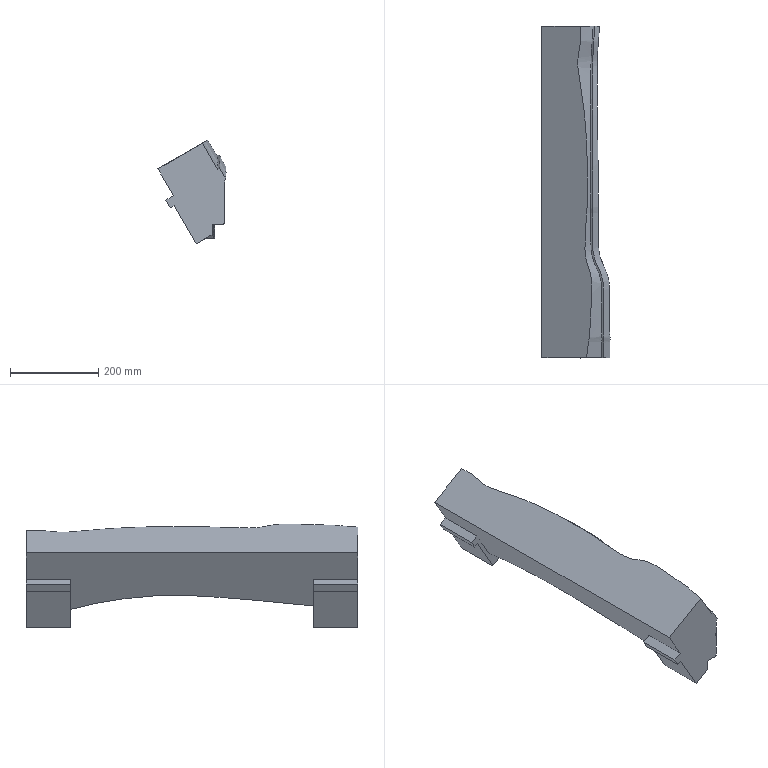Part | NX | features solid 2 | 1 solid | 62 faces | box 154.017 x 750 x 234.81 mm | volume 11650363 mm3 | spline 44 | plane 18